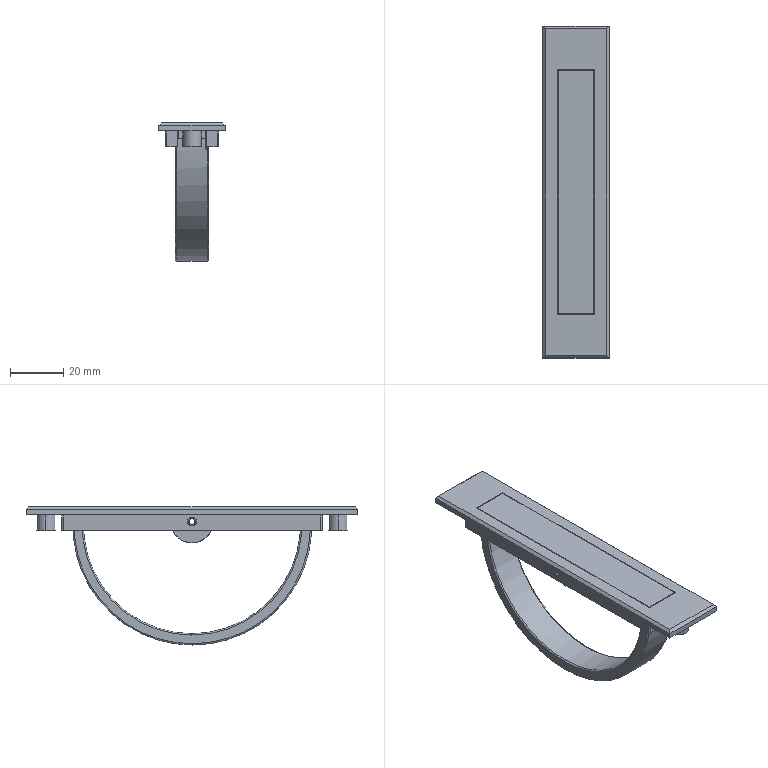Part | NX | features BREP 2 | 2 solids | 128 faces | box 25 x 125 x 52 mm | volume 23535 mm3 | plane 66 | cylinder 40 | torus 14 | cone 8 | commonest cylinder face diameters 2 x8 1 x6 3 x4 3.242 x4 3.3 x4 7 x4